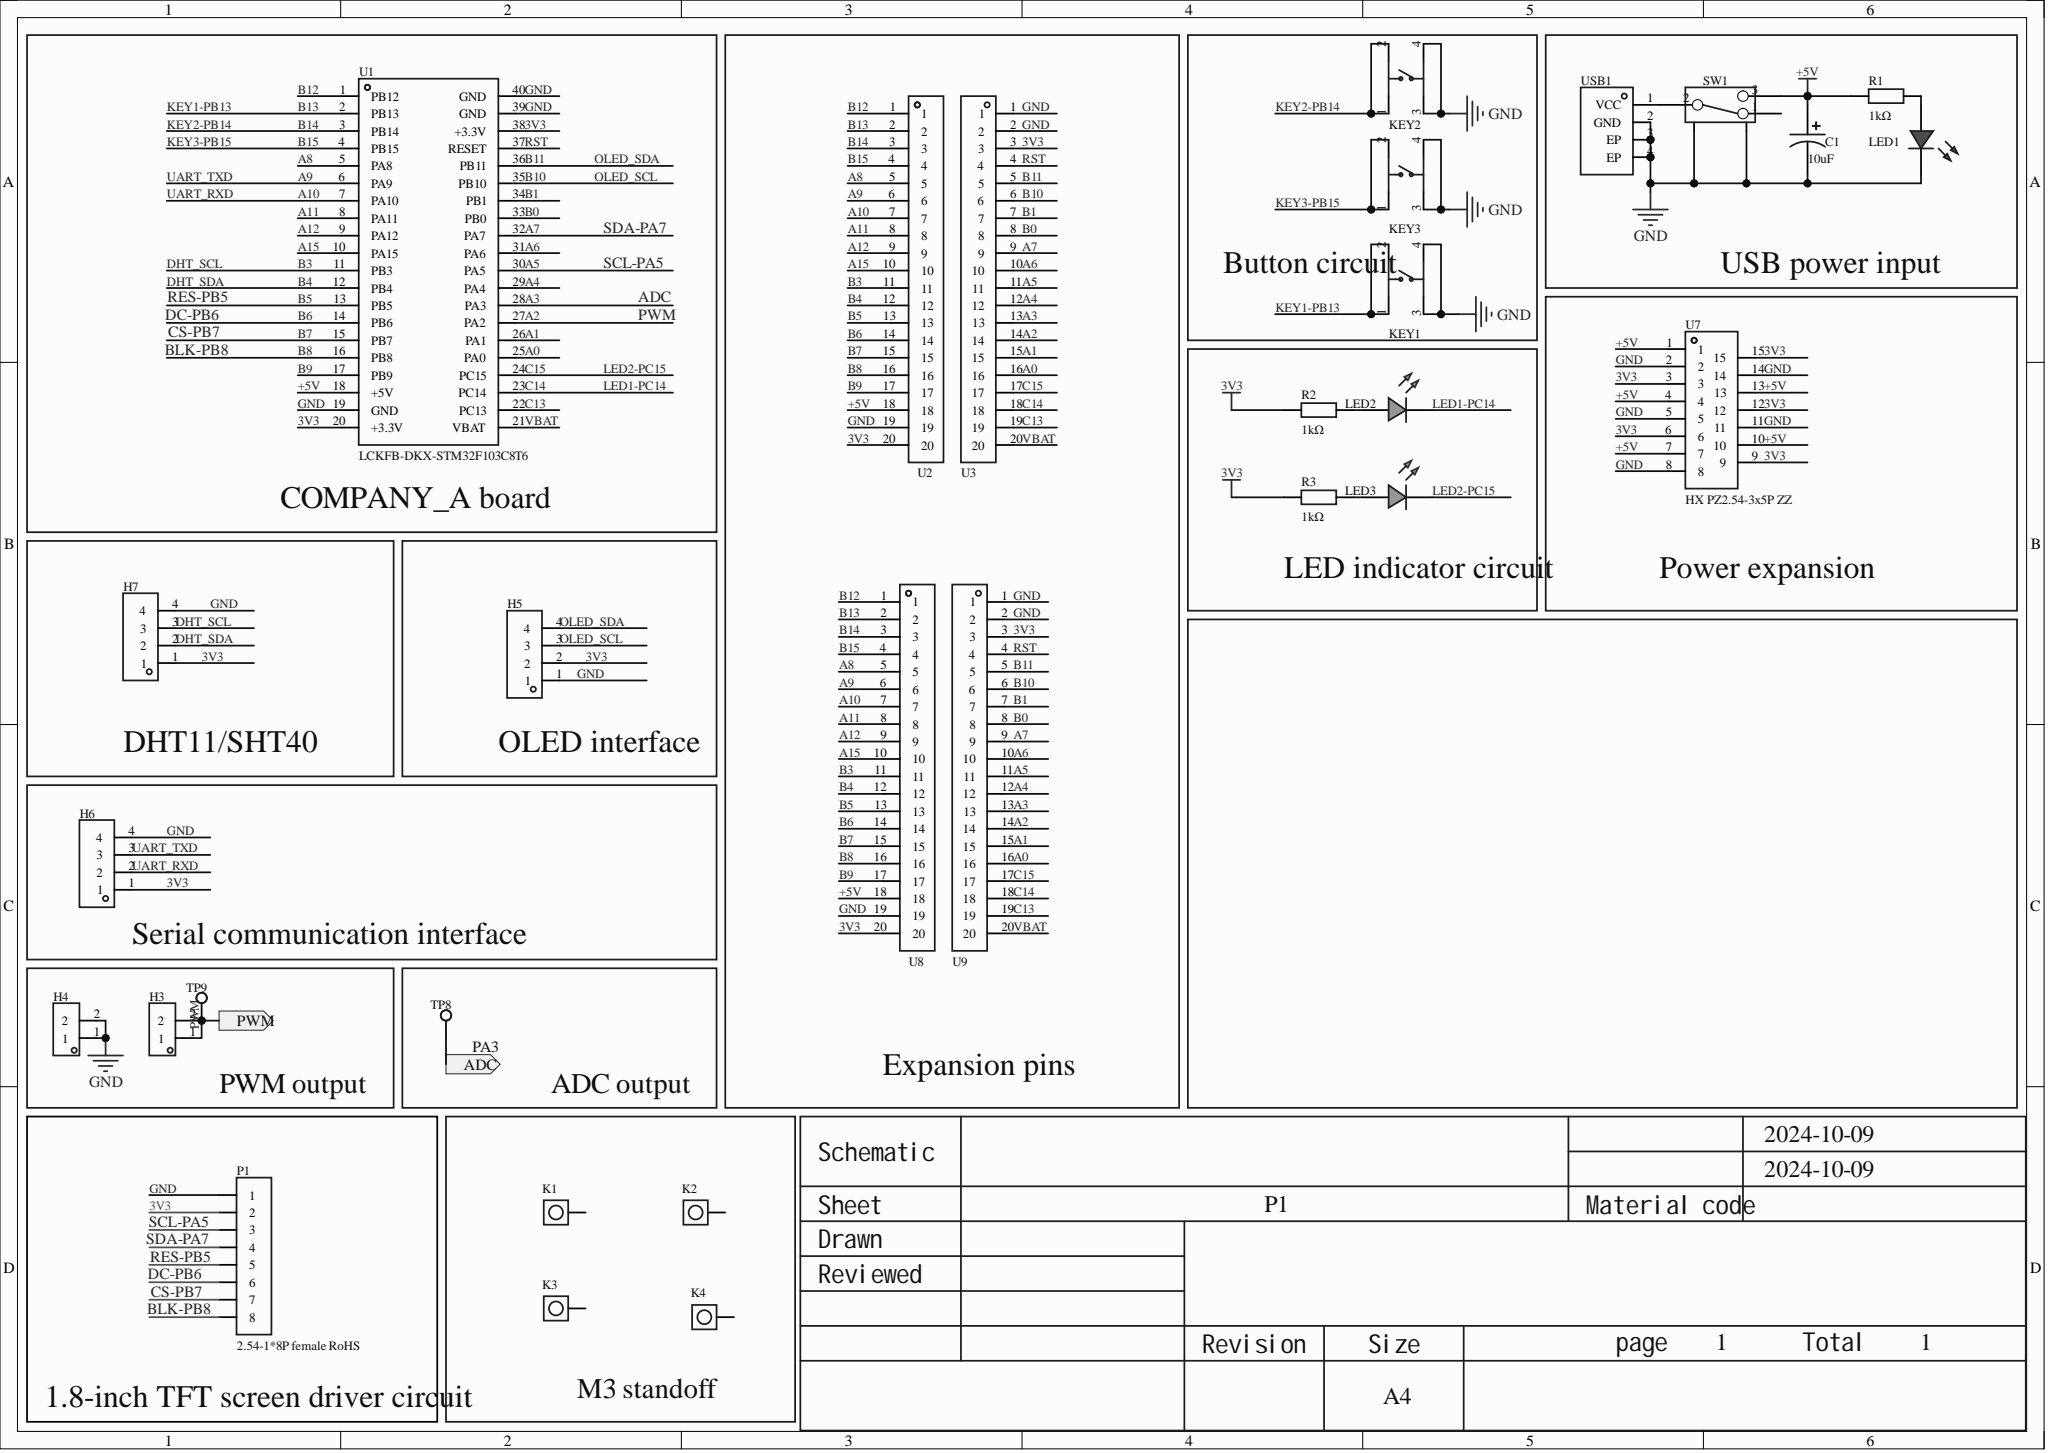Circuit board | Altium Designer | 30 parts | 41 nets
Bill of materials:
Comment,Description,Designator,Footprint,LibRef,Quantity
"01EC1809SHC10UF50V","Capacitance: 10uF; tolerance: ±20%; rated voltage: 50V; ripple current: 50mA@120Hz; ESR: -;","C1","CAP-TH_BD5.0-P2.00-D0.8-FD","01EC1809SHC10UF50V","1"
"HDR-M_2.54_1x2P","","H3, H4","HDR-TH_2P-P2.54-V-M-1","HDR-M_2.54_1x2P","2"
"2.54-1*4P female","Socket structure: 1x4P; pitch: 2.54mm; row spacing: -; round/square hole: square hole; mounting type: through-hole; rows: single row; total positions: 4P; rated current: 3A; rated voltage: -; socket direction: top; height: -; contact material: bronze; contact plating: -; operating temperature: -40℃~+105℃; soldering temperature (max): -;","H5, H6, H7","HDR-TH_4P-P2.54-V-F","2.54-1*4P母","3"
"Flange pad","","K1, K2, K3, K4","法兰焊盘-8孔-M3","法兰焊盘-8孔-M3","4"
"TC-6610-9-260G","Contact current: 50mA; rated voltage (AC): -; rated voltage (DC): 12V; rated power: -; insulation resistance: -; circuit: SPST; mounting style: upright SMD; with LED: -; actuating force: -; mechanical life: 10 wan cycles; with bracket: No;","KEY1, KEY2, KEY3","SW-TH_4P-L5.0-W5.0-P4.50-LS6.5","TC-6610-9-260G","3"
"LED_TH-R_3mm","","LED1","LED_TH-3mm","LED_TH-R_3mm","1"
"LED_TH-G_3mm","","LED2, LED3","LED_TH-3mm","LED_TH-G_3mm","2"
"2.54-1*8P female RoHS","Socket structure: 1x8P; pitch: 2.54mm; row spacing: -; mounting type: through-hole; rows: single row; total positions: 8P; height: -; contact material: -; contact plating: -;","P1","HDR-TH_8P-P2.54-V-F-1","2.54-1*8P母环保","1"
"MFR0W4F1001A50","Resistor type: metal film resistor; resistance: 1kΩ; tolerance: ±1%; power: 250mW; temperature coefficient: ±50ppm/?;","R1, R2, R3","RES-TH_BD2.5-L6.5-P10.50-D0.6","MFR0W4F1001A50","3"
"SK-12E12-G5","Rated current (DC): -; rated voltage (DC): -; rated current (AC): -; rated voltage (AC): -; circuit: SPDT; mounting style: horizontal insertion; mechanical life: 5 thousand cycles;","SW1","SW-TH_SK-12E12-G5","SK-12E12-G5","1"
"TP-yellow test point","","TP8, TP9","TESTPOINT-TH_BD3.2","TP-黄色测试点","2"
"LCKFB-DKX-STM32F103C8T6","","U1","CONN-TH_L53.3-W22.9_STM32F103C8T6-CARD","LCKFB-DKX-STM32F103C8T6","1"
"KH-2.54FH-1X20P-H8.5","Socket structure: 1x20P; pitch: 2.54mm; row spacing: -; round/square hole: square hole; mounting type: through-hole; rows: single row; total positions: 20P; rated current: 3A; rated voltage: -; socket direction: top; height: 8.5mm; operating temperature: -40℃~+105℃;","U2, U3, U8, U9","HDR-TH_20P-P2.54-V-F-2","KH-2.54FH-1X20P-H8.5","4"
"HX PZ2.54-3x5P ZZ","Pin structure: 3x5P; pitch: 2.54mm; row spacing: -; round/square pin: square pin; mounting type: through-hole; rows: three rows; total pins: 15P; rated current: 3A; rated voltage: 1kV; mating pin length: 3mm; height: 2.5mm; tail length: 6mm; contact material: brass; contact plating: gold; operating temperature: -40℃~+105℃; soldering temperature (max): 260℃;","U7","HDR-TH_15P-P2.54-V-M-R3-C5-S7.5","HX PZ2.54-3x5P ZZ","1"
"KH-TYPE-C-2P","Connector type: -; standard: -; male/female: -; number of contacts: -; number of ports: -; mounting type: -; rated current - power: -; contact material: -; contact plating: -; operating temperature range: -;","USB1","USB-SMD_KH-TYPE-C-2P","KH-TYPE-C-2P","1"
Netlist (Protel format):
[
C1
CAP-TH_BD5.0-P2.00-D0.8-FD
01EC1809SHC10UF50V



]
[
H3
HDR-TH_2P-P2.54-V-M-1
HDR-M_2.54_1x2P



]
[
H4
HDR-TH_2P-P2.54-V-M-1
HDR-M_2.54_1x2P



]
[
H5
HDR-TH_4P-P2.54-V-F
2.54-1*4P female



]
[
H6
HDR-TH_4P-P2.54-V-F
2.54-1*4P female



]
[
H7
HDR-TH_4P-P2.54-V-F
2.54-1*4P female



]
[
K1
法兰焊盘-8孔-M3
Flange pad



]
[
K2
法兰焊盘-8孔-M3
Flange pad



]
[
K3
法兰焊盘-8孔-M3
Flange pad



]
[
K4
法兰焊盘-8孔-M3
Flange pad



]
[
KEY1
SW-TH_4P-L5.0-W5.0-P4.50-LS6.5
TC-6610-9-260G



]
[
KEY2
SW-TH_4P-L5.0-W5.0-P4.50-LS6.5
TC-6610-9-260G



]
[
KEY3
SW-TH_4P-L5.0-W5.0-P4.50-LS6.5
TC-6610-9-260G



]
[
LED1
LED_TH-3mm
LED_TH-R_3mm



]
[
LED2
LED_TH-3mm
LED_TH-G_3mm



]
[
LED3
LED_TH-3mm
LED_TH-G_3mm



]
[
P1
HDR-TH_8P-P2.54-V-F-1
2.54-1*8P female RoHS



]
[
R1
RES-TH_BD2.5-L6.5-P10.50-D0.6
MFR0W4F1001A50



]
[
R2
RES-TH_BD2.5-L6.5-P10.50-D0.6
MFR0W4F1001A50



]
[
R3
RES-TH_BD2.5-L6.5-P10.50-D0.6
MFR0W4F1001A50



]
[
SW1
SW-TH_SK-12E12-G5
SK-12E12-G5



]
[
TP8
TESTPOINT-TH_BD3.2
TP-yellow test point



]
[
TP9
TESTPOINT-TH_BD3.2
TP-yellow test point



]
[
U1
CONN-TH_L53.3-W22.9_STM32F103C8T6-CARD
LCKFB-DKX-STM32F103C8T6



]
[
U2
HDR-TH_20P-P2.54-V-F-2
KH-2.54FH-1X20P-H8.5



]
[
U3
HDR-TH_20P-P2.54-V-F-2
KH-2.54FH-1X20P-H8.5



]
[
U7
HDR-TH_15P-P2.54-V-M-R3-C5-S7.5
HX PZ2.54-3x5P ZZ



]
[
U8
HDR-TH_20P-P2.54-V-F-2
KH-2.54FH-1X20P-H8.5



]
[
U9
HDR-TH_20P-P2.54-V-F-2
KH-2.54FH-1X20P-H8.5



]
[
USB1
USB-SMD_KH-TYPE-C-2P
KH-TYPE-C-2P



]
(
VBAT
U1-21
U3-20
U9-20
)
(
RST
U1-37
U3-4
U9-4
)
(
NetSW1_2
SW1-2
USB1-1
)
(
NetLED3_1
LED3-1
R3-1
)
(
NetLED2_1
LED2-1
R2-1
)
(
NetLED1_1
LED1-1
R1-1
)
(
GND
C1-2
H4-1
H4-2
H5-1
H6-4
H7-4
KEY1-3
KEY1-4
KEY2-3
KEY2-4
KEY3-3
KEY3-4
LED1-2
P1-1
SW1-4
SW1-5
U1-19
U1-39
U1-40
U2-19
U3-1
U3-2
U7-2
U7-5
U7-8
U7-11
U7-14
U8-19
U9-1
U9-2
USB1-2
USB1-3
USB1-4
)
(
C15
LED3-2
U1-24
U3-17
U9-17
)
(
C14
LED2-2
U1-23
U3-18
U9-18
)
(
C13
U1-22
U3-19
U9-19
)
(
B15
KEY3-1
KEY3-2
U1-4
U2-4
U8-4
)
(
B14
KEY2-1
KEY2-2
U1-3
U2-3
U8-3
)
(
B13
KEY1-1
KEY1-2
U1-2
U2-2
U8-2
)
(
B12
U1-1
U2-1
U8-1
)
(
B11
H5-4
U1-36
U3-5
U9-5
)
(
B10
H5-3
U1-35
U3-6
U9-6
)
(
B9
U1-17
U2-17
U8-17
)
(
B8
P1-8
U1-16
U2-16
U8-16
)
(
B7
P1-7
U1-15
U2-15
U8-15
)
(
B6
P1-6
U1-14
U2-14
U8-14
)
(
B5
P1-5
U1-13
U2-13
U8-13
)
(
B4
H7-2
U1-12
U2-12
U8-12
)
(
B3
H7-3
U1-11
U2-11
U8-11
)
(
B1
U1-34
U3-7
U9-7
)
(
B0
U1-33
U3-8
U9-8
)
(
A15
U1-10
U2-10
U8-10
)
(
A12
U1-9
U2-9
U8-9
)
(
A11
U1-8
U2-8
U8-8
)
(
A10
H6-2
U1-7
U2-7
U8-7
)
(
A9
H6-3
U1-6
U2-6
U8-6
)
(
A8
U1-5
U2-5
U8-5
)
(
A7
P1-4
U1-32
U3-9
U9-9
)
(
A6
U1-31
U3-10
U9-10
)
(
A5
P1-3
U1-30
U3-11
U9-11
)
(
A4
U1-29
U3-12
U9-12
)
(
A3
U1-28
U3-13
U9-13
)
(
A2
H3-1
H3-2
TP9-1
U1-27
U3-14
U9-14
)
(
A1
U1-26
U3-15
U9-15
)
(
A0
U1-25
U3-16
U9-16
)
(
+5V
C1-1
R1-2
SW1-3
U1-18
U2-18
U7-1
U7-4
U7-7
U7-10
U7-13
U8-18
)
(
3V3
H5-2
H6-1
H7-1
P1-2
R2-2
R3-2
U1-20
U1-38
U2-20
U3-3
U7-3
U7-6
U7-9
U7-12
U7-15
U8-20
U9-3
)